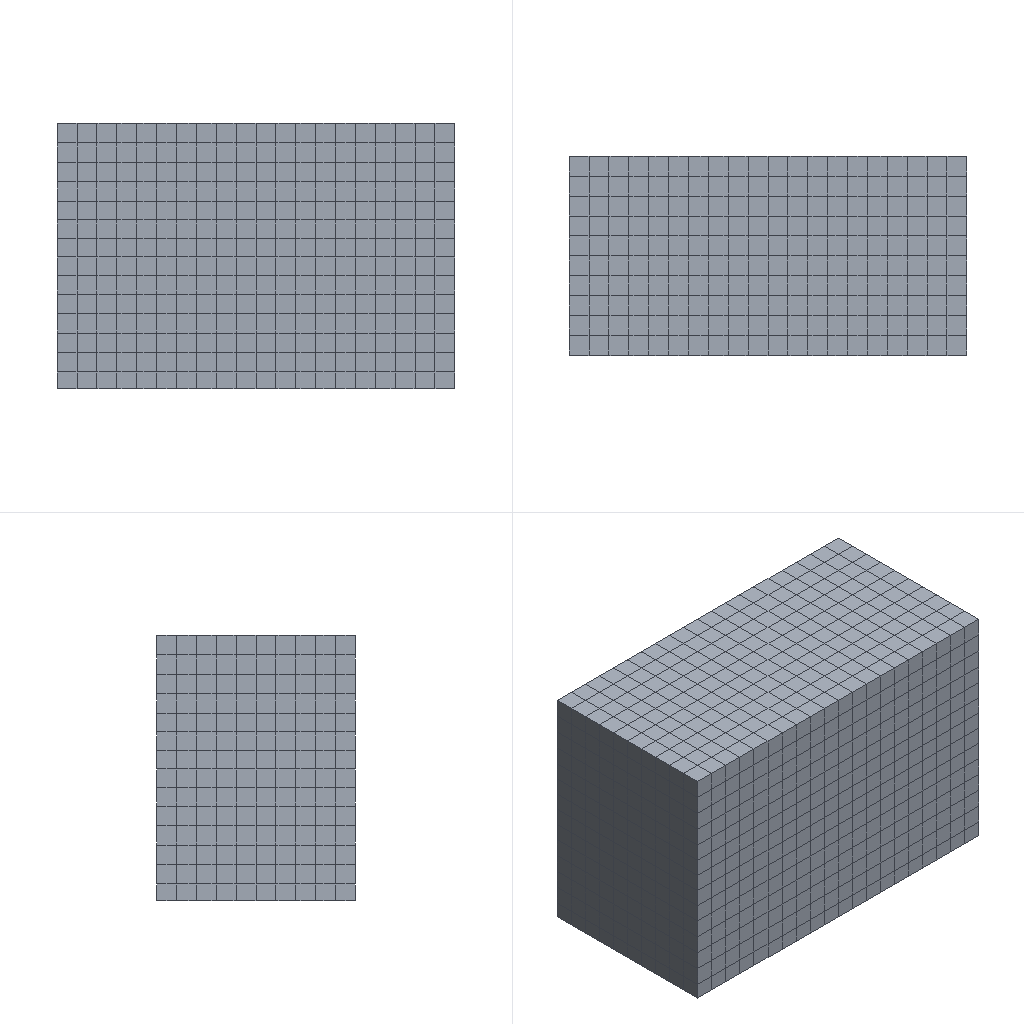Simulation study | abaqus
Set-up summary:
category,name,step,type,value,unit,region
solver,abaqus
solver,version,,,Abaqus/Standard 2020
units,not stated in the deck,,not stated
analysis,deck,,soils,soils
load_step,Step-1,Step-1,soils
load_step,requested,,,1
mesh,nodes,,,3465
mesh,elements,,,2800
element_type,C3D8RP,,solid,2800
load,load commands in deck,,count,1
bc,support commands in deck,,count,4
material,SHA,,in results
material,SOIL,,in results
check,setup vs results,,match,"per instance, exact: element labels, types and connectivity; labels of the nodes the elements use; coordinates of those nodes at SINGLE_PRECISION in 1 of 1 instance(s)"
Abaqus input file, long lists of numbers shortened:
*Heading
** Job name: Job-1 Model name: Model-1
** Generated by: Abaqus/CAE 2020
*Preprint, echo=NO, model=NO, history=NO, contact=NO
**
** PARTS
**
*Part, name=Part-1
*Node
      1,   1.2,           0.,  0.565
      2,   1.2, -0.6,  0.565
** (3463 more lines like these left out)
*Element, type=C3D8RP
   1,  110,  565, 1756,  413,    1,   21,  341,   46
   2,  565,  566, 1757, 1756,   21,   22,  342,  341
** (2798 more lines like these left out)
*Nset, nset=Set-1
    1,    2,    3,    4,    5,    6,    7,    8,    9,   10,   11,   12,   13,   14,   15,   16
   21,   22,   23,   24,   25,   26,   27,   28,   29,   30,   31,   32,   33,   34,   35,   36
** (201 more lines like these left out)
*Elset, elset=Set-1, generate
    1,  2600,     1
*Nset, nset=Set-2
   13,   14,   15,   16,   17,   18,   19,   20,  220,  221,  222,  223,  224,  225,  226,  227
  228,  235,  236,  237,  238,  239,  240,  241,  242,  243,  247,  248,  249,  250,  251,  252
** (27 more lines like these left out)
*Elset, elset=Set-2, generate
 2601,  2800,     1
*Orientation, name=Ori-1
1., 0., 0., 0., 1., 0.
1, 0.
** Section: soil
*Solid Section, elset=Set-1, orientation=Ori-1, material=soil
,
** Section: sha
*Solid Section, elset=Set-2, orientation=Ori-1, material=sha
,
*End Part
**
**
** ASSEMBLY
**
*Assembly, name=Assembly
**
*Instance, name=Part-1-1, part=Part-1
*End Instance
**
*Nset, nset=Set-1, instance=Part-1-1
    1,    2,    3,    4,    5,    6,    7,    8,    9,   10,   11,   12,   13,   14,   15,   16
   17,   18,   19,   20,   30,   31,   32,   33,   43,   44,   45,   46,   56,   57,   58,   59
** (38 more lines like these left out)
*Elset, elset=Set-1, instance=Part-1-1
    1,   10,   11,   20,   21,   30,   31,   40,   41,   50,   51,   60,   61,   70,   71,   80
   81,   90,   91,  100,  101,  110,  111,  120,  121,  130,  131,  140,  141,  150,  151,  160
** (33 more lines like these left out)
*Nset, nset=Set-2, instance=Part-1-1
    1,    2,    3,    4,    5,    6,    7,    8,    9,   10,   11,   12,   13,   14,   15,   16
   17,   18,   19,   20,   21,   22,   23,   24,   25,   26,   27,   28,   29,   30,   31,   32
** (19 more lines like these left out)
*Elset, elset=Set-2, instance=Part-1-1
    1,    2,    3,    4,    5,    6,    7,    8,    9,   10,   11,   12,   13,   14,   15,   16
   17,   18,   19,   20,   21,   22,   23,   24,   25,   26,   27,   28,   29,   30,   31,   32
** (16 more lines like these left out)
*Nset, nset=Set-3, instance=Part-1-1
   17,   18,   19,   20,  285,  286,  287,  288,  289,  290,  291,  292,  293,  294,  295,  296
  297,  298,  299,  300,  301,  302,  303,  304,  305,  306,  307,  308,  309,  310,  311,  312
** (13 more lines like these left out)
*Elset, elset=Set-3, instance=Part-1-1, generate
 2601,  2800,     1
*Nset, nset=Set-4, instance=Part-1-1
   17,   18,   19,   20,  285,  286,  287,  288,  289,  290,  291,  292,  293,  294,  295,  296
  297,  298,  299,  300,  301,  302,  303,  304,  305,  306,  307,  308,  309,  310,  311,  312
** (13 more lines like these left out)
*Elset, elset=Set-4, instance=Part-1-1, generate
 2601,  2800,     1
*Nset, nset=Set-5, instance=Part-1-1, generate
    1,  3465,     1
*Elset, elset=Set-5, instance=Part-1-1, generate
    1,  2800,     1
*Nset, nset=Set-6, instance=Part-1-1, generate
    1,  3465,     1
*Elset, elset=Set-6, instance=Part-1-1, generate
    1,  2800,     1
*Nset, nset=Set-7, instance=Part-1-1
    1,    2,    3,    4,    5,    6,    7,    8,    9,   10,   11,   12,   13,   14,   15,   16
   17,   18,   19,   20,   21,   22,   23,   24,   25,   26,   27,   28,   29,   34,   35,   36
** (157 more lines like these left out)
*Elset, elset=Set-7, instance=Part-1-1, generate
 1001,  2800,     1
*Nset, nset=Set-8, instance=Part-1-1
    1,    2,    3,    4,    5,    6,    7,    8,   21,   22,   23,   24,   25,   26,   27,   28
   29,   30,   31,   32,   33,   34,   35,   36,   37,   38,   39,   40,   41,   42,   43,   44
** (85 more lines like these left out)
*Elset, elset=Set-8, instance=Part-1-1, generate
    1,  1000,     1
*Nset, nset=Set-9, instance=Part-1-1
    1,    2,    5,    8,    9,   10,   11,   12,   21,   22,   23,   24,   25,   26,   27,   28
   29,   47,   48,   49,   50,   51,   52,   53,   54,   55,   92,   93,   94,   95,   96,   97
** (71 more lines like these left out)
*Elset, elset=Set-9, instance=Part-1-1, generate
 1001,  1800,     1
*Nset, nset=Set-10, instance=Part-1-1
    1,    2,    3,    4,    5,    6,    7,    8,   13,   14,   15,   16,   17,   18,   19,   20
   21,   22,   23,   24,   25,   26,   27,   28,   29,   30,   31,   32,   33,   34,   35,   36
** (157 more lines like these left out)
*Elset, elset=Set-10, instance=Part-1-1
    1,    2,    3,    4,    5,    6,    7,    8,    9,   10,   11,   12,   13,   14,   15,   16
   17,   18,   19,   20,   21,   22,   23,   24,   25,   26,   27,   28,   29,   30,   31,   32
** (123 more lines like these left out)
*Elset, elset=_Surf-1_S5, internal, instance=Part-1-1
 1031, 1032, 1033, 1034, 1035, 1036, 1037, 1038, 1039, 1040, 1071, 1072, 1073, 1074, 1075, 1076
 1077, 1078, 1079, 1080, 1111, 1112, 1113, 1114, 1115, 1116, 1117, 1118, 1119, 1120, 1151, 1152
** (11 more lines like these left out)
*Surface, type=ELEMENT, name=Surf-1
_Surf-1_S5, S5
*Nset, nset=Set-4_PP_, internal, instance=Part-1-1
   17,   18,   19,   20,  285,  286,  287,  288,  289,  290,  291,  292,  293,  294,  295,  296
  297,  298,  299,  300,  301,  302,  303,  304,  305,  306,  307,  308,  309,  310,  311,  312
** (13 more lines like these left out)
*End Assembly
*Amplitude, name=Amp-1
             0.,              0.,            100.,              1.
**
** MATERIALS
**
*Material, name=sha
*Elastic
 1.5e+07, 0.2
*Gap Flow
 0.001,
*Permeability, specific=9800., type=ORTHOTROPIC
 2.5e-07, 2.5e-07, 2.3e-07,     0.1
*Material, name=soil
*Elastic
 1.45e+06, 0.38
*Gap Flow
 0.001,
*Permeability, specific=9800., type=ORTHOTROPIC
 5.07e-09, 5.07e-09, 3.72e-09,     0.05
*Mohr Coulomb
 11.4, 0.1
*Mohr Coulomb Hardening
9320.,0.
**
** PREDEFINED FIELDS
**
** Name: Predefined Field-1   Type: Void ratio
*Initial Conditions, TYPE=RATIO
Set-5, 0.2
** Name: Predefined Field-2   Type: Pore pressure
*Initial Conditions, TYPE=PORE PRESSURE
Set-9, 500000.
** Name: Predefined Field-middle Type: [REDACTED] [REDACTED]
*Initial Conditions, TYPE=PORE PRESSURE
Set-10, 5e+09
** ----------------------------------------------------------------
**
** STEP: Step-1
**
*Step, name=Step-1, nlgeom=YES, inc=10000, unsymm=YES
*Soils, consolidation, end=PERIOD, utol=1e+19, stabilize=0.0002, allsdtol=0.05, continue=NO
1., 1.2096e+06, 0.1, 1.2096e+06,
**
** BOUNDARY CONDITIONS
**
** Name: BC-1 Type: 位移/转角
*Boundary
Set-1, 2, 2
** Name: BC-2 Type: 位移/转角
*Boundary
Set-2, 1, 1
** Name: BC-3 Type: 位移/转角
*Boundary
Set-3, 3, 3
** Name: [REDACTED] : Pore pressure
*Boundary
Set-4_PP_, 8, 8
**
** LOADS
**
** Name: Load-1   Type: Pressure
*Dsload, amplitude=Amp-1
Surf-1, P, 5000.
**
** OUTPUT REQUESTS
**
*Restart, write, frequency=0
**
** FIELD OUTPUT: F-Output-1
**
*Output, field
*Node Output
POR, RF, RT, U, V
*Element Output, directions=YES
E, FLUVR, FLVEL, LE, MISES, MISESMAX, PE, PEEQ, PEEQMAX, PEEQT, PEMAG, PEQC, S, SAT, VE, VEEQ
VOIDR
*Output, history, frequency=0
*End Step
Results summary:
result,step,,completed,increments=31 time=1209600.0/1209600.0
result,analysis,,,"soils, consolidation"
result,last_loadstep,,,1
result,primary field,,,"U, POR"
result,reaction total,,FX,0.0,model units
result,reaction total,,FY,0.0,model units
result,reaction total,,FZ,3600,model units